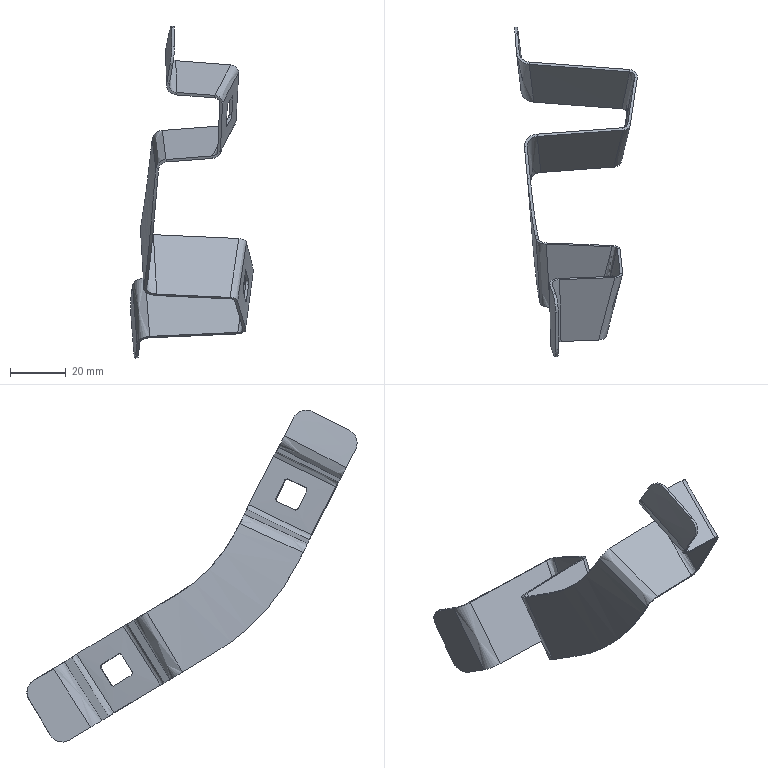Part | STEP file | FNA5401837 | 1 solid | 94 faces | box 44.202 x 118.87 x 119.505 mm | volume 6315 mm3 | spline 94